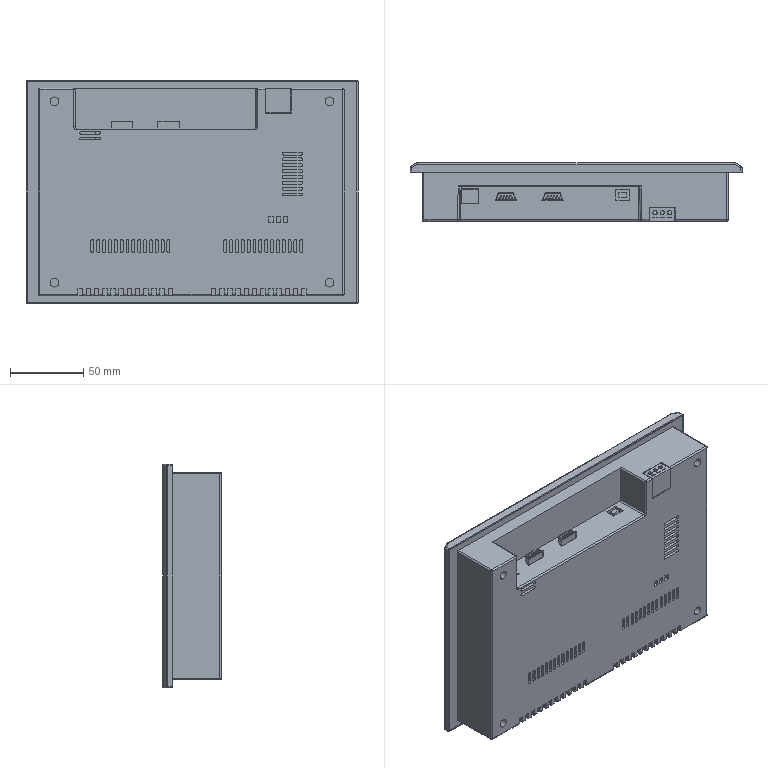Part | SolidWorks | features BaseBody 27 | 27 solids | 849 faces | box 227 x 40.02 x 153 mm | volume 206698 mm3 | plane 539 | cylinder 189 | spline 85 | cone 36 | commonest cylinder face diameters 2 x159 6 x10 10 x8 2.8 x6 3 x6